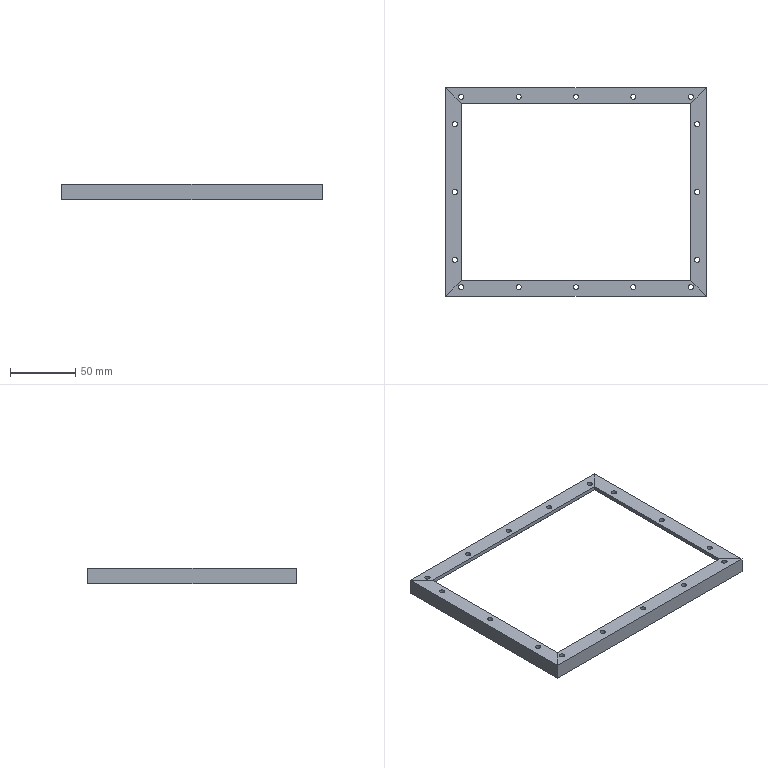Part | STEP file | 1-43.4 | 1 solid | 40 faces | box 200 x 160 x 12 mm | volume 42705 mm3 | plane 24 | cylinder 16 | commonest cylinder face diameters 4 x16